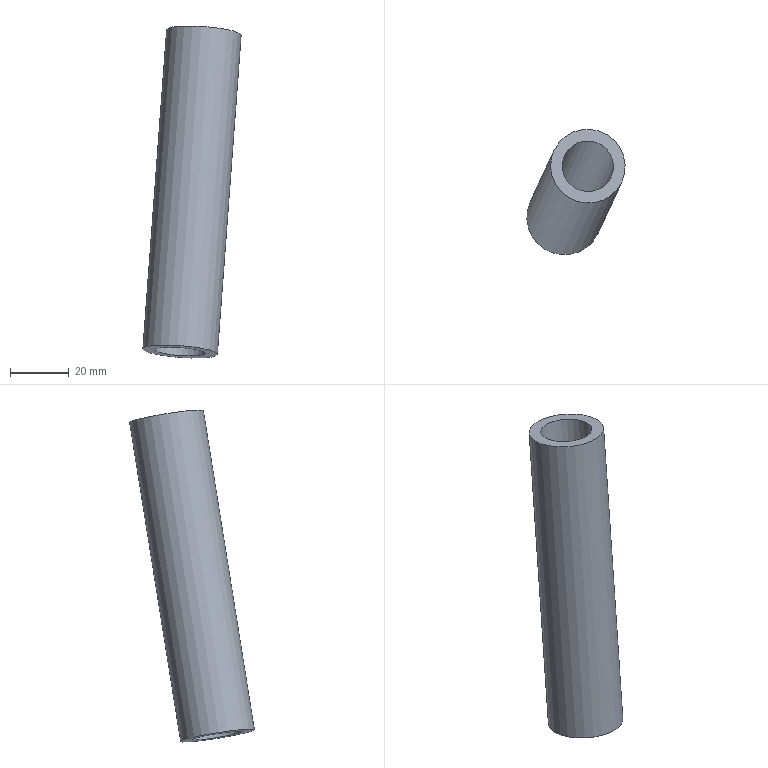Part | NX | features solid 2 | 1 solid | 4 faces | box 33.404 x 42.395 x 112.74 mm | volume 29581 mm3 | plane 2 | cylinder 2 | commonest cylinder face diameters 17.4 x1 25.4 x1
STEP:
#1=CARTESIAN_POINT('',(448.986,561.072,108.14));
#2=VERTEX_POINT('',#1);
#3=CARTESIAN_POINT('',(460.496,555.705,108.14));
#4=DIRECTION('',(0.07339,0.1574,0.9848));
#5=DIRECTION('',(-0.9063,0.4226,-0.000000001));
#6=AXIS2_PLACEMENT_3D('',#3,#4,#5);
#7=CIRCLE('',#6,12.7);
#8=EDGE_CURVE('',#2,#2,#7,.F.);
#9=ORIENTED_EDGE('',*,*,#8,.T.);
#10=EDGE_LOOP('',(#9));
#11=FACE_BOUND('',#10,.T.);
#12=CARTESIAN_POINT('',(452.611,559.382,108.14));
#13=VERTEX_POINT('',#12);
#14=CARTESIAN_POINT('',(460.496,555.705,108.14));
#15=DIRECTION('',(0.07339,0.1574,0.9848));
#16=DIRECTION('',(-0.9063,0.4226,-0.000000001));
#17=AXIS2_PLACEMENT_3D('',#14,#15,#16);
#18=CIRCLE('',#17,8.7);
#19=EDGE_CURVE('',#13,#13,#18,.F.);
#20=ORIENTED_EDGE('',*,*,#19,.F.);
#21=EDGE_LOOP('',(#20));
#22=FACE_BOUND('',#21,.T.);
#23=CARTESIAN_POINT('',(460.496,555.705,108.14));
#24=DIRECTION('',(-0.07339,-0.1574,-0.9848));
#25=DIRECTION('',(-0.9063,0.4226,-0.000000001));
#26=AXIS2_PLACEMENT_3D('',#23,#24,#25);
#27=PLANE('',#26);
#28=ADVANCED_FACE('',(#11,#22),#27,.T.);
#29=CARTESIAN_POINT('',(457.058,578.384,216.468));
#30=VERTEX_POINT('',#29);
#31=CARTESIAN_POINT('',(468.568,573.017,216.468));
#32=DIRECTION('',(0.07339,0.1574,0.9848));
#33=DIRECTION('',(-0.9063,0.4226,-0.000000001));
#34=AXIS2_PLACEMENT_3D('',#31,#32,#33);
#35=CIRCLE('',#34,12.7);
#36=EDGE_CURVE('',#30,#30,#35,.F.);
#37=ORIENTED_EDGE('',*,*,#36,.F.);
#38=EDGE_LOOP('',(#37));
#39=FACE_BOUND('',#38,.T.);
#40=CARTESIAN_POINT('',(476.453,569.34,216.468));
#41=VERTEX_POINT('',#40);
#42=CARTESIAN_POINT('',(468.568,573.017,216.468));
#43=DIRECTION('',(-0.07339,-0.1574,-0.9848));
#44=DIRECTION('',(0.9063,-0.4226,0.000000001));
#45=AXIS2_PLACEMENT_3D('',#42,#43,#44);
#46=CIRCLE('',#45,8.7);
#47=EDGE_CURVE('',#41,#41,#46,.T.);
#48=ORIENTED_EDGE('',*,*,#47,.T.);
#49=EDGE_LOOP('',(#48));
#50=FACE_BOUND('',#49,.T.);
#51=CARTESIAN_POINT('',(468.568,573.017,216.468));
#52=DIRECTION('',(-0.07339,-0.1574,-0.9848));
#53=DIRECTION('',(-0.9063,0.4226,-0.000000001));
#54=AXIS2_PLACEMENT_3D('',#51,#52,#53);
#55=PLANE('',#54);
#56=ADVANCED_FACE('',(#39,#50),#55,.F.);
#57=ORIENTED_EDGE('',*,*,#8,.F.);
#58=EDGE_LOOP('',(#57));
#59=FACE_BOUND('',#58,.T.);
#60=ORIENTED_EDGE('',*,*,#36,.T.);
#61=EDGE_LOOP('',(#60));
#62=FACE_BOUND('',#61,.T.);
#63=CARTESIAN_POINT('',(468.568,573.017,216.468));
#64=DIRECTION('',(-0.07339,-0.1574,-0.9848));
#65=DIRECTION('',(-0.9063,0.4226,-0.000000001));
#66=AXIS2_PLACEMENT_3D('',#63,#64,#65);
#67=CYLINDRICAL_SURFACE('',#66,12.7);
#68=ADVANCED_FACE('',(#59,#62),#67,.T.);
#69=ORIENTED_EDGE('',*,*,#19,.T.);
#70=EDGE_LOOP('',(#69));
#71=FACE_BOUND('',#70,.T.);
#72=ORIENTED_EDGE('',*,*,#47,.F.);
#73=EDGE_LOOP('',(#72));
#74=FACE_BOUND('',#73,.T.);
#75=CARTESIAN_POINT('',(468.568,573.017,216.468));
#76=DIRECTION('',(-0.07339,-0.1574,-0.9848));
#77=DIRECTION('',(-0.9063,0.4226,-0.000000001));
#78=AXIS2_PLACEMENT_3D('',#75,#76,#77);
#79=CYLINDRICAL_SURFACE('',#78,8.7);
#80=ADVANCED_FACE('',(#71,#74),#79,.F.);
#81=CLOSED_SHELL('',(#28,#56,#68,#80));
#82=MANIFOLD_SOLID_BREP('',#81);
#83=(LENGTH_UNIT()NAMED_UNIT(*)SI_UNIT(.MILLI.,.METRE.));
#84=UNCERTAINTY_MEASURE_WITH_UNIT(LENGTH_MEASURE(0.00001),#83,'','');
#85=(NAMED_UNIT(*)PLANE_ANGLE_UNIT()SI_UNIT($,.RADIAN.));
#86=(NAMED_UNIT(*)SI_UNIT($,.STERADIAN.)SOLID_ANGLE_UNIT());
#87=(GEOMETRIC_REPRESENTATION_CONTEXT(3)GLOBAL_UNCERTAINTY_ASSIGNED_CONTEXT((#84))GLOBAL_UNIT_ASSIGNED_CONTEXT((#83,#85,#86))REPRESENTATION_CONTEXT('',''));
#88=ADVANCED_BREP_SHAPE_REPRESENTATION('',(#82),#87);